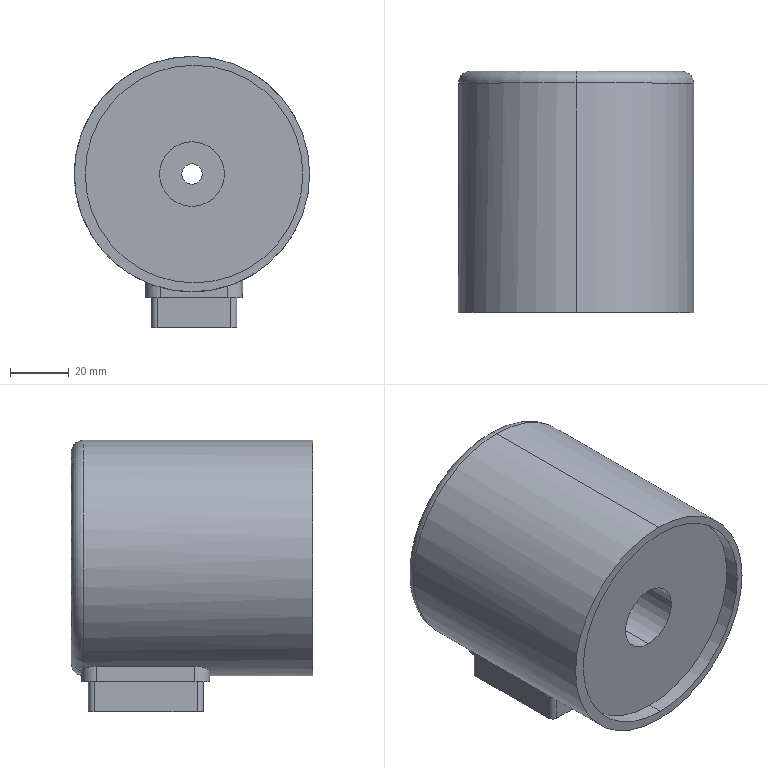Part | STEP file | 1 solid | 36 faces | box 80 x 82 x 92.2 mm | volume 393243 mm3 | cylinder 18 | plane 16 | torus 2 | commonest cylinder face diameters 4 x4 10 x4 80 x4 7 x2 22 x2 74 x2
STEP:
#1=CARTESIAN_POINT('',(0.,-31.446,37.));
#2=VERTEX_POINT('',#1);
#3=CARTESIAN_POINT('',(0.,-31.446,-37.));
#4=VERTEX_POINT('',#3);
#5=CARTESIAN_POINT('',(0.,-31.446,0.));
#6=DIRECTION('',(0.,-1.,0.));
#7=DIRECTION('',(0.,0.,-1.));
#8=AXIS2_PLACEMENT_3D('',#5,#6,#7);
#9=CIRCLE('',#8,37.);
#10=EDGE_CURVE('',#2,#4,#9,.T.);
#11=ORIENTED_EDGE('',*,*,#10,.F.);
#12=CARTESIAN_POINT('',(0.,-36.446,37.));
#13=VERTEX_POINT('',#12);
#14=CARTESIAN_POINT('',(0.,-31.446,37.));
#15=DIRECTION('',(0.,-1.,0.));
#16=VECTOR('',#15,1000.);
#17=LINE('',#14,#16);
#18=EDGE_CURVE('',#2,#13,#17,.T.);
#19=ORIENTED_EDGE('',*,*,#18,.T.);
#20=CARTESIAN_POINT('',(0.,-36.446,-37.));
#21=VERTEX_POINT('',#20);
#22=CARTESIAN_POINT('',(0.,-36.446,0.));
#23=DIRECTION('',(0.,-1.,0.));
#24=DIRECTION('',(0.,0.,-1.));
#25=AXIS2_PLACEMENT_3D('',#22,#23,#24);
#26=CIRCLE('',#25,37.);
#27=EDGE_CURVE('',#13,#21,#26,.T.);
#28=ORIENTED_EDGE('',*,*,#27,.T.);
#29=CARTESIAN_POINT('',(0.,-31.446,-37.));
#30=DIRECTION('',(0.,-1.,0.));
#31=VECTOR('',#30,1000.);
#32=LINE('',#29,#31);
#33=EDGE_CURVE('',#4,#21,#32,.T.);
#34=ORIENTED_EDGE('',*,*,#33,.F.);
#35=EDGE_LOOP('',(#11,#19,#28,#34));
#36=FACE_OUTER_BOUND('',#35,.T.);
#37=CARTESIAN_POINT('',(0.,-31.446,0.));
#38=DIRECTION('',(0.,-1.,0.));
#39=DIRECTION('',(0.,0.,-1.));
#40=AXIS2_PLACEMENT_3D('',#37,#38,#39);
#41=CYLINDRICAL_SURFACE('',#40,37.);
#42=ADVANCED_FACE('',(#36),#41,.F.);
#43=CARTESIAN_POINT('',(13.564,41.554,-37.37));
#44=VERTEX_POINT('',#43);
#45=CARTESIAN_POINT('',(-0.7,41.554,40.));
#46=VERTEX_POINT('',#45);
#47=CARTESIAN_POINT('',(-0.7,41.554,0.));
#48=DIRECTION('',(0.,-1.,0.));
#49=DIRECTION('',(0.,0.,-1.));
#50=AXIS2_PLACEMENT_3D('',#47,#48,#49);
#51=CIRCLE('',#50,40.);
#52=EDGE_CURVE('',#44,#46,#51,.T.);
#53=ORIENTED_EDGE('',*,*,#52,.T.);
#54=CARTESIAN_POINT('',(-0.7,-36.446,40.));
#55=VERTEX_POINT('',#54);
#56=CARTESIAN_POINT('',(-0.7,-36.446,40.));
#57=DIRECTION('',(0.,-1.,0.));
#58=VECTOR('',#57,1000.);
#59=LINE('',#56,#58);
#60=EDGE_CURVE('',#46,#55,#59,.T.);
#61=ORIENTED_EDGE('',*,*,#60,.T.);
#62=CARTESIAN_POINT('',(-0.7,-36.446,-40.));
#63=VERTEX_POINT('',#62);
#64=CARTESIAN_POINT('',(-0.7,-36.446,0.));
#65=DIRECTION('',(0.,-1.,0.));
#66=DIRECTION('',(0.,0.,-1.));
#67=AXIS2_PLACEMENT_3D('',#64,#65,#66);
#68=CIRCLE('',#67,40.);
#69=EDGE_CURVE('',#63,#55,#68,.T.);
#70=ORIENTED_EDGE('',*,*,#69,.F.);
#71=CARTESIAN_POINT('',(-0.7,-1.446,-40.));
#72=VERTEX_POINT('',#71);
#73=CARTESIAN_POINT('',(-0.7,-36.446,-40.));
#74=DIRECTION('',(0.,-1.,0.));
#75=VECTOR('',#74,1000.);
#76=LINE('',#73,#75);
#77=EDGE_CURVE('',#72,#63,#76,.T.);
#78=ORIENTED_EDGE('',*,*,#77,.F.);
#79=CARTESIAN_POINT('',(11.5,-1.446,-38.094));
#80=VERTEX_POINT('',#79);
#81=CARTESIAN_POINT('',(-0.7,-1.446,0.));
#82=DIRECTION('',(0.,-1.,0.));
#83=DIRECTION('',(1.,0.,0.));
#84=AXIS2_PLACEMENT_3D('',#81,#82,#83);
#85=CIRCLE('',#84,40.);
#86=EDGE_CURVE('',#72,#80,#85,.T.);
#87=ORIENTED_EDGE('',*,*,#86,.T.);
#88=CARTESIAN_POINT('',(16.5,3.554,-36.113));
#89=VERTEX_POINT('',#88);
#90=CARTESIAN_POINT('',(11.5,-1.446,-38.094));
#91=CARTESIAN_POINT('',(12.145,-1.446,-37.888));
#92=CARTESIAN_POINT('',(12.785,-1.321,-37.664));
#93=CARTESIAN_POINT('',(13.528,-1.019,-37.384));
#94=CARTESIAN_POINT('',(13.673,-0.9519,-37.329));
#95=CARTESIAN_POINT('',(13.956,-0.8041,-37.218));
#96=CARTESIAN_POINT('',(14.093,-0.7245,-37.165));
#97=CARTESIAN_POINT('',(14.365,-0.5472,-37.055));
#98=CARTESIAN_POINT('',(14.496,-0.4525,-37.001));
#99=CARTESIAN_POINT('',(14.748,-0.2509,-36.897));
#100=CARTESIAN_POINT('',(14.868,-0.1449,-36.846));
#101=CARTESIAN_POINT('',(15.102,0.08269,-36.746));
#102=CARTESIAN_POINT('',(15.213,0.2015,-36.699));
#103=CARTESIAN_POINT('',(15.37,0.3872,-36.63));
#104=CARTESIAN_POINT('',(15.421,0.4504,-36.608));
#105=CARTESIAN_POINT('',(15.52,0.5792,-36.564));
#106=CARTESIAN_POINT('',(15.566,0.6431,-36.543));
#107=CARTESIAN_POINT('',(15.709,0.8492,-36.48));
#108=CARTESIAN_POINT('',(15.796,0.9903,-36.44));
#109=CARTESIAN_POINT('',(15.956,1.28,-36.367));
#110=CARTESIAN_POINT('',(16.029,1.428,-36.334));
#111=CARTESIAN_POINT('',(16.161,1.736,-36.273));
#112=CARTESIAN_POINT('',(16.219,1.893,-36.246));
#113=CARTESIAN_POINT('',(16.294,2.132,-36.21));
#114=CARTESIAN_POINT('',(16.317,2.212,-36.2));
#115=CARTESIAN_POINT('',(16.359,2.374,-36.18));
#116=CARTESIAN_POINT('',(16.378,2.453,-36.171));
#117=CARTESIAN_POINT('',(16.465,2.873,-36.13));
#118=CARTESIAN_POINT('',(16.5,3.212,-36.113));
#119=CARTESIAN_POINT('',(16.5,3.554,-36.113));
#120=B_SPLINE_CURVE_WITH_KNOTS('',3,(#90,#91,#92,#93,#94,#95,#96,#97,#98,#99,#100,#101,#102,#103,#104,#105,#106,#107,#108,#109,#110,#111,#112,#113,#114,#115,#116,#117,#118,#119),.UNSPECIFIED.,.F.,.F.,(4,2,2,2,2,2,2,2,2,2,2,2,2,2,4),(0.,0.25,0.3125,0.375,0.4375,0.5,0.5625,0.5938,0.625,0.6875,0.75,0.8125,0.8438,0.875,1.),.UNSPECIFIED.);
#121=EDGE_CURVE('',#80,#89,#120,.T.);
#122=ORIENTED_EDGE('',*,*,#121,.T.);
#123=CARTESIAN_POINT('',(16.5,37.,-36.113));
#124=VERTEX_POINT('',#123);
#125=CARTESIAN_POINT('',(16.5,-36.446,-36.113));
#126=DIRECTION('',(0.,1.,0.));
#127=VECTOR('',#126,1000.);
#128=LINE('',#125,#127);
#129=EDGE_CURVE('',#89,#124,#128,.T.);
#130=ORIENTED_EDGE('',*,*,#129,.T.);
#131=CARTESIAN_POINT('',(16.5,37.,-36.113));
#132=CARTESIAN_POINT('',(16.5,37.246,-36.113));
#133=CARTESIAN_POINT('',(16.482,37.49,-36.122));
#134=CARTESIAN_POINT('',(16.429,37.851,-36.147));
#135=CARTESIAN_POINT('',(16.395,38.031,-36.163));
#136=CARTESIAN_POINT('',(16.352,38.21,-36.183));
#137=CARTESIAN_POINT('',(16.321,38.328,-36.198));
#138=CARTESIAN_POINT('',(16.304,38.389,-36.206));
#139=CARTESIAN_POINT('',(16.216,38.678,-36.247));
#140=CARTESIAN_POINT('',(16.13,38.903,-36.287));
#141=CARTESIAN_POINT('',(15.978,39.229,-36.357));
#142=CARTESIAN_POINT('',(15.895,39.389,-36.395));
#143=CARTESIAN_POINT('',(15.804,39.546,-36.437));
#144=CARTESIAN_POINT('',(15.741,39.649,-36.465));
#145=CARTESIAN_POINT('',(15.708,39.702,-36.48));
#146=CARTESIAN_POINT('',(15.545,39.949,-36.553));
#147=CARTESIAN_POINT('',(15.401,40.136,-36.617));
#148=CARTESIAN_POINT('',(15.168,40.401,-36.718));
#149=CARTESIAN_POINT('',(15.046,40.529,-36.771));
#150=CARTESIAN_POINT('',(14.917,40.651,-36.825));
#151=CARTESIAN_POINT('',(14.83,40.731,-36.862));
#152=CARTESIAN_POINT('',(14.784,40.771,-36.882));
#153=CARTESIAN_POINT('',(14.383,41.112,-37.049));
#154=CARTESIAN_POINT('',(13.992,41.36,-37.207));
#155=CARTESIAN_POINT('',(13.564,41.554,-37.37));
#156=B_SPLINE_CURVE_WITH_KNOTS('',3,(#131,#132,#133,#134,#135,#136,#137,#138,#139,#140,#141,#142,#143,#144,#145,#146,#147,#148,#149,#150,#151,#152,#153,#154,#155),.UNSPECIFIED.,.F.,.F.,(4,2,1,2,2,2,1,2,2,2,1,2,2,4),(0.,0.125,0.1875,0.2188,0.25,0.375,0.4375,0.4688,0.5,0.625,0.6875,0.7188,0.75,1.),.UNSPECIFIED.);
#157=EDGE_CURVE('',#124,#44,#156,.T.);
#158=ORIENTED_EDGE('',*,*,#157,.T.);
#159=EDGE_LOOP('',(#53,#61,#70,#78,#87,#122,#130,#158));
#160=FACE_OUTER_BOUND('',#159,.T.);
#161=CARTESIAN_POINT('',(-0.7,-36.446,0.));
#162=DIRECTION('',(0.,-1.,0.));
#163=DIRECTION('',(0.,0.,-1.));
#164=AXIS2_PLACEMENT_3D('',#161,#162,#163);
#165=CYLINDRICAL_SURFACE('',#164,40.);
#166=ADVANCED_FACE('',(#160),#165,.T.);
#167=CARTESIAN_POINT('',(-0.7,45.554,-36.));
#168=VERTEX_POINT('',#167);
#169=CARTESIAN_POINT('',(-0.7,45.554,36.));
#170=VERTEX_POINT('',#169);
#171=CARTESIAN_POINT('',(-0.7,45.554,0.));
#172=DIRECTION('',(0.,-1.,0.));
#173=DIRECTION('',(0.,0.,-1.));
#174=AXIS2_PLACEMENT_3D('',#171,#172,#173);
#175=CIRCLE('',#174,36.);
#176=EDGE_CURVE('',#168,#170,#175,.T.);
#177=ORIENTED_EDGE('',*,*,#176,.T.);
#178=CARTESIAN_POINT('',(-0.7,41.554,36.));
#179=DIRECTION('',(1.,0.,0.));
#180=DIRECTION('',(0.,0.,-1.));
#181=AXIS2_PLACEMENT_3D('',#178,#179,#180);
#182=CIRCLE('',#181,4.);
#183=EDGE_CURVE('',#170,#46,#182,.T.);
#184=ORIENTED_EDGE('',*,*,#183,.T.);
#185=ORIENTED_EDGE('',*,*,#52,.F.);
#186=CARTESIAN_POINT('',(11.79,41.554,-38.));
#187=VERTEX_POINT('',#186);
#188=CARTESIAN_POINT('',(-0.7,41.554,0.));
#189=DIRECTION('',(0.,-1.,0.));
#190=DIRECTION('',(0.,0.,-1.));
#191=AXIS2_PLACEMENT_3D('',#188,#189,#190);
#192=CIRCLE('',#191,40.);
#193=EDGE_CURVE('',#187,#44,#192,.T.);
#194=ORIENTED_EDGE('',*,*,#193,.F.);
#195=CARTESIAN_POINT('',(11.711,41.996,-38.));
#196=VERTEX_POINT('',#195);
#197=CARTESIAN_POINT('',(11.711,41.996,-38.));
#198=CARTESIAN_POINT('',(11.737,41.925,-38.));
#199=CARTESIAN_POINT('',(11.756,41.853,-38.));
#200=CARTESIAN_POINT('',(11.783,41.703,-38.));
#201=CARTESIAN_POINT('',(11.79,41.629,-38.));
#202=CARTESIAN_POINT('',(11.79,41.554,-38.));
#203=B_SPLINE_CURVE_WITH_KNOTS('',3,(#197,#198,#199,#200,#201,#202),.UNSPECIFIED.,.F.,.F.,(4,2,4),(0.01192,0.01214,0.01237),.UNSPECIFIED.);
#204=EDGE_CURVE('',#196,#187,#203,.T.);
#205=ORIENTED_EDGE('',*,*,#204,.F.);
#206=CARTESIAN_POINT('',(11.5,42.,-38.068));
#207=VERTEX_POINT('',#206);
#208=CARTESIAN_POINT('',(11.711,41.996,-38.));
#209=CARTESIAN_POINT('',(11.641,41.999,-38.023));
#210=CARTESIAN_POINT('',(11.571,42.,-38.045));
#211=CARTESIAN_POINT('',(11.5,42.,-38.068));
#212=B_SPLINE_CURVE_WITH_KNOTS('',3,(#208,#209,#210,#211),.UNSPECIFIED.,.F.,.F.,(4,4),(0.000000653,0.0002228),.UNSPECIFIED.);
#213=EDGE_CURVE('',#196,#207,#212,.T.);
#214=ORIENTED_EDGE('',*,*,#213,.T.);
#215=CARTESIAN_POINT('',(-0.7,42.,-39.975));
#216=VERTEX_POINT('',#215);
#217=CARTESIAN_POINT('',(-0.7,42.,0.));
#218=DIRECTION('',(0.,1.,0.));
#219=DIRECTION('',(0.,0.,-1.));
#220=AXIS2_PLACEMENT_3D('',#217,#218,#219);
#221=CIRCLE('',#220,39.975);
#222=EDGE_CURVE('',#207,#216,#221,.T.);
#223=ORIENTED_EDGE('',*,*,#222,.T.);
#224=CARTESIAN_POINT('',(-0.7,41.554,-36.));
#225=DIRECTION('',(-1.,0.,0.));
#226=DIRECTION('',(0.,0.,1.));
#227=AXIS2_PLACEMENT_3D('',#224,#225,#226);
#228=CIRCLE('',#227,4.);
#229=EDGE_CURVE('',#168,#216,#228,.T.);
#230=ORIENTED_EDGE('',*,*,#229,.F.);
#231=EDGE_LOOP('',(#177,#184,#185,#194,#205,#214,#223,#230));
#232=FACE_OUTER_BOUND('',#231,.T.);
#233=CARTESIAN_POINT('',(-0.7,41.554,0.));
#234=DIRECTION('',(0.,-1.,0.));
#235=DIRECTION('',(0.,0.,-1.));
#236=AXIS2_PLACEMENT_3D('',#233,#234,#235);
#237=TOROIDAL_SURFACE('',#236,36.,4.);
#238=ADVANCED_FACE('',(#232),#237,.T.);
#239=CARTESIAN_POINT('',(2.8,-3.446,0.));
#240=VERTEX_POINT('',#239);
#241=CARTESIAN_POINT('',(-4.2,-3.446,0.));
#242=VERTEX_POINT('',#241);
#243=CARTESIAN_POINT('',(-0.7,-3.446,0.));
#244=DIRECTION('',(0.,1.,0.));
#245=DIRECTION('',(0.,0.,-1.));
#246=AXIS2_PLACEMENT_3D('',#243,#244,#245);
#247=CIRCLE('',#246,3.5);
#248=EDGE_CURVE('',#240,#242,#247,.T.);
#249=ORIENTED_EDGE('',*,*,#248,.F.);
#250=CARTESIAN_POINT('',(2.8,45.554,0.));
#251=VERTEX_POINT('',#250);
#252=CARTESIAN_POINT('',(2.8,-60.446,0.));
#253=DIRECTION('',(0.,1.,0.));
#254=VECTOR('',#253,1000.);
#255=LINE('',#252,#254);
#256=EDGE_CURVE('',#240,#251,#255,.T.);
#257=ORIENTED_EDGE('',*,*,#256,.T.);
#258=CARTESIAN_POINT('',(-4.2,45.554,0.));
#259=VERTEX_POINT('',#258);
#260=CARTESIAN_POINT('',(-0.7,45.554,0.));
#261=DIRECTION('',(0.,1.,0.));
#262=DIRECTION('',(-1.,0.,0.));
#263=AXIS2_PLACEMENT_3D('',#260,#261,#262);
#264=CIRCLE('',#263,3.5);
#265=EDGE_CURVE('',#251,#259,#264,.T.);
#266=ORIENTED_EDGE('',*,*,#265,.T.);
#267=CARTESIAN_POINT('',(-4.2,-60.446,0.));
#268=DIRECTION('',(0.,1.,0.));
#269=VECTOR('',#268,1000.);
#270=LINE('',#267,#269);
#271=EDGE_CURVE('',#242,#259,#270,.T.);
#272=ORIENTED_EDGE('',*,*,#271,.F.);
#273=EDGE_LOOP('',(#249,#257,#266,#272));
#274=FACE_OUTER_BOUND('',#273,.T.);
#275=CARTESIAN_POINT('',(-0.7,-60.446,0.));
#276=DIRECTION('',(0.,1.,0.));
#277=DIRECTION('',(-1.,0.,0.));
#278=AXIS2_PLACEMENT_3D('',#275,#276,#277);
#279=CYLINDRICAL_SURFACE('',#278,3.5);
#280=ADVANCED_FACE('',(#274),#279,.F.);
#281=CARTESIAN_POINT('',(-0.7,-3.446,11.));
#282=VERTEX_POINT('',#281);
#283=CARTESIAN_POINT('',(-0.7,-3.446,-11.));
#284=VERTEX_POINT('',#283);
#285=CARTESIAN_POINT('',(-0.7,-3.446,0.));
#286=DIRECTION('',(0.,-1.,0.));
#287=DIRECTION('',(0.,0.,-1.));
#288=AXIS2_PLACEMENT_3D('',#285,#286,#287);
#289=CIRCLE('',#288,11.);
#290=EDGE_CURVE('',#282,#284,#289,.T.);
#291=ORIENTED_EDGE('',*,*,#290,.F.);
#292=CARTESIAN_POINT('',(-0.7,-31.446,11.));
#293=VERTEX_POINT('',#292);
#294=CARTESIAN_POINT('',(-0.7,-3.446,11.));
#295=DIRECTION('',(0.,-1.,0.));
#296=VECTOR('',#295,1000.);
#297=LINE('',#294,#296);
#298=EDGE_CURVE('',#282,#293,#297,.T.);
#299=ORIENTED_EDGE('',*,*,#298,.T.);
#300=CARTESIAN_POINT('',(-0.7,-31.446,-11.));
#301=VERTEX_POINT('',#300);
#302=CARTESIAN_POINT('',(-0.7,-31.446,0.));
#303=DIRECTION('',(0.,1.,0.));
#304=DIRECTION('',(0.,0.,-1.));
#305=AXIS2_PLACEMENT_3D('',#302,#303,#304);
#306=CIRCLE('',#305,11.);
#307=EDGE_CURVE('',#301,#293,#306,.T.);
#308=ORIENTED_EDGE('',*,*,#307,.F.);
#309=CARTESIAN_POINT('',(-0.7,-3.446,-11.));
#310=DIRECTION('',(0.,-1.,0.));
#311=VECTOR('',#310,1000.);
#312=LINE('',#309,#311);
#313=EDGE_CURVE('',#284,#301,#312,.T.);
#314=ORIENTED_EDGE('',*,*,#313,.F.);
#315=EDGE_LOOP('',(#291,#299,#308,#314));
#316=FACE_OUTER_BOUND('',#315,.T.);
#317=CARTESIAN_POINT('',(-0.7,-3.446,0.));
#318=DIRECTION('',(0.,-1.,0.));
#319=DIRECTION('',(0.,0.,-1.));
#320=AXIS2_PLACEMENT_3D('',#317,#318,#319);
#321=CYLINDRICAL_SURFACE('',#320,11.);
#322=ADVANCED_FACE('',(#316),#321,.F.);
#323=CARTESIAN_POINT('',(16.5,37.,-42.));
#324=VERTEX_POINT('',#323);
#325=CARTESIAN_POINT('',(16.5,3.554,-42.));
#326=VERTEX_POINT('',#325);
#327=CARTESIAN_POINT('',(16.5,3.554,-42.));
#328=DIRECTION('',(0.,-1.,0.));
#329=VECTOR('',#328,1000.);
#330=LINE('',#327,#329);
#331=EDGE_CURVE('',#324,#326,#330,.T.);
#332=ORIENTED_EDGE('',*,*,#331,.T.);
#333=CARTESIAN_POINT('',(11.5,-1.446,-42.));
#334=VERTEX_POINT('',#333);
#335=CARTESIAN_POINT('',(11.5,3.554,-42.));
#336=DIRECTION('',(0.,0.,-1.));
#337=DIRECTION('',(1.,0.,0.));
#338=AXIS2_PLACEMENT_3D('',#335,#336,#337);
#339=CIRCLE('',#338,5.);
#340=EDGE_CURVE('',#326,#334,#339,.T.);
#341=ORIENTED_EDGE('',*,*,#340,.T.);
#342=CARTESIAN_POINT('',(-11.5,-1.446,-42.));
#343=VERTEX_POINT('',#342);
#344=CARTESIAN_POINT('',(11.5,-1.446,-42.));
#345=DIRECTION('',(-1.,0.,0.));
#346=VECTOR('',#345,1000.);
#347=LINE('',#344,#346);
#348=EDGE_CURVE('',#334,#343,#347,.T.);
#349=ORIENTED_EDGE('',*,*,#348,.T.);
#350=CARTESIAN_POINT('',(-16.5,3.554,-42.));
#351=VERTEX_POINT('',#350);
#352=CARTESIAN_POINT('',(-11.5,3.554,-42.));
#353=DIRECTION('',(0.,0.,-1.));
#354=DIRECTION('',(1.,0.,0.));
#355=AXIS2_PLACEMENT_3D('',#352,#353,#354);
#356=CIRCLE('',#355,5.);
#357=EDGE_CURVE('',#343,#351,#356,.T.);
#358=ORIENTED_EDGE('',*,*,#357,.T.);
#359=CARTESIAN_POINT('',(-16.5,37.,-42.));
#360=VERTEX_POINT('',#359);
#361=CARTESIAN_POINT('',(-16.5,37.,-42.));
#362=DIRECTION('',(0.,1.,0.));
#363=VECTOR('',#362,1000.);
#364=LINE('',#361,#363);
#365=EDGE_CURVE('',#351,#360,#364,.T.);
#366=ORIENTED_EDGE('',*,*,#365,.T.);
#367=CARTESIAN_POINT('',(-11.5,42.,-42.));
#368=VERTEX_POINT('',#367);
#369=CARTESIAN_POINT('',(-11.5,37.,-42.));
#370=DIRECTION('',(0.,0.,-1.));
#371=DIRECTION('',(1.,0.,0.));
#372=AXIS2_PLACEMENT_3D('',#369,#370,#371);
#373=CIRCLE('',#372,5.);
#374=EDGE_CURVE('',#360,#368,#373,.T.);
#375=ORIENTED_EDGE('',*,*,#374,.T.);
#376=CARTESIAN_POINT('',(11.5,42.,-42.));
#377=VERTEX_POINT('',#376);
#378=CARTESIAN_POINT('',(-11.5,42.,-42.));
#379=DIRECTION('',(1.,0.,0.));
#380=VECTOR('',#379,1000.);
#381=LINE('',#378,#380);
#382=EDGE_CURVE('',#368,#377,#381,.T.);
#383=ORIENTED_EDGE('',*,*,#382,.T.);
#384=CARTESIAN_POINT('',(11.5,37.,-42.));
#385=DIRECTION('',(0.,0.,-1.));
#386=DIRECTION('',(1.,0.,0.));
#387=AXIS2_PLACEMENT_3D('',#384,#385,#386);
#388=CIRCLE('',#387,5.);
#389=EDGE_CURVE('',#377,#324,#388,.T.);
#390=ORIENTED_EDGE('',*,*,#389,.T.);
#391=EDGE_LOOP('',(#332,#341,#349,#358,#366,#375,#383,#390));
#392=FACE_OUTER_BOUND('',#391,.T.);
#393=CARTESIAN_POINT('',(-12.5,0.777,-42.));
#394=VERTEX_POINT('',#393);
#395=CARTESIAN_POINT('',(-14.5,2.777,-42.));
#396=VERTEX_POINT('',#395);
#397=CARTESIAN_POINT('',(-12.5,2.777,-42.));
#398=DIRECTION('',(0.,0.,-1.));
#399=DIRECTION('',(-1.,0.,0.));
#400=AXIS2_PLACEMENT_3D('',#397,#398,#399);
#401=CIRCLE('',#400,2.);
#402=EDGE_CURVE('',#394,#396,#401,.T.);
#403=ORIENTED_EDGE('',*,*,#402,.F.);
#404=CARTESIAN_POINT('',(12.5,0.777,-42.));
#405=VERTEX_POINT('',#404);
#406=CARTESIAN_POINT('',(12.5,0.777,-42.));
#407=DIRECTION('',(-1.,0.,0.));
#408=VECTOR('',#407,1000.);
#409=LINE('',#406,#408);
#410=EDGE_CURVE('',#405,#394,#409,.T.);
#411=ORIENTED_EDGE('',*,*,#410,.F.);
#412=CARTESIAN_POINT('',(14.5,2.777,-42.));
#413=VERTEX_POINT('',#412);
#414=CARTESIAN_POINT('',(12.5,2.777,-42.));
#415=DIRECTION('',(0.,0.,-1.));
#416=DIRECTION('',(1.,0.,0.));
#417=AXIS2_PLACEMENT_3D('',#414,#415,#416);
#418=CIRCLE('',#417,2.);
#419=EDGE_CURVE('',#413,#405,#418,.T.);
#420=ORIENTED_EDGE('',*,*,#419,.F.);
#421=CARTESIAN_POINT('',(14.5,37.777,-42.));
#422=VERTEX_POINT('',#421);
#423=CARTESIAN_POINT('',(14.5,2.777,-42.));
#424=DIRECTION('',(0.,-1.,0.));
#425=VECTOR('',#424,1000.);
#426=LINE('',#423,#425);
#427=EDGE_CURVE('',#422,#413,#426,.T.);
#428=ORIENTED_EDGE('',*,*,#427,.F.);
#429=CARTESIAN_POINT('',(12.5,39.777,-42.));
#430=VERTEX_POINT('',#429);
#431=CARTESIAN_POINT('',(12.5,37.777,-42.));
#432=DIRECTION('',(0.,0.,-1.));
#433=DIRECTION('',(1.,0.,0.));
#434=AXIS2_PLACEMENT_3D('',#431,#432,#433);
#435=CIRCLE('',#434,2.);
#436=EDGE_CURVE('',#430,#422,#435,.T.);
#437=ORIENTED_EDGE('',*,*,#436,.F.);
#438=CARTESIAN_POINT('',(-12.5,39.777,-42.));
#439=VERTEX_POINT('',#438);
#440=CARTESIAN_POINT('',(12.5,39.777,-42.));
#441=DIRECTION('',(1.,0.,0.));
#442=VECTOR('',#441,1000.);
#443=LINE('',#440,#442);
#444=EDGE_CURVE('',#439,#430,#443,.T.);
#445=ORIENTED_EDGE('',*,*,#444,.F.);
#446=CARTESIAN_POINT('',(-14.5,37.777,-42.));
#447=VERTEX_POINT('',#446);
#448=CARTESIAN_POINT('',(-12.5,37.777,-42.));
#449=DIRECTION('',(0.,0.,-1.));
#450=DIRECTION('',(1.,0.,0.));
#451=AXIS2_PLACEMENT_3D('',#448,#449,#450);
#452=CIRCLE('',#451,2.);
#453=EDGE_CURVE('',#447,#439,#452,.T.);
#454=ORIENTED_EDGE('',*,*,#453,.F.);
#455=CARTESIAN_POINT('',(-14.5,2.777,-42.));
#456=DIRECTION('',(0.,1.,0.));
#457=VECTOR('',#456,1000.);
#458=LINE('',#455,#457);
#459=EDGE_CURVE('',#396,#447,#458,.T.);
#460=ORIENTED_EDGE('',*,*,#459,.F.);
#461=EDGE_LOOP('',(#403,#411,#420,#428,#437,#445,#454,#460));
#462=FACE_BOUND('',#461,.T.);
#463=CARTESIAN_POINT('',(11.5,37.,-42.));
#464=DIRECTION('',(0.,0.,1.));
#465=DIRECTION('',(1.,0.,0.));
#466=AXIS2_PLACEMENT_3D('',#463,#464,#465);
#467=PLANE('',#466);
#468=ADVANCED_FACE('',(#392,#462),#467,.F.);
#469=ORIENTED_EDGE('',*,*,#298,.F.);
#470=CARTESIAN_POINT('',(-0.7,-3.446,0.));
#471=DIRECTION('',(0.,-1.,0.));
#472=DIRECTION('',(0.,0.,-1.));
#473=AXIS2_PLACEMENT_3D('',#470,#471,#472);
#474=CIRCLE('',#473,11.);
#475=EDGE_CURVE('',#284,#282,#474,.T.);
#476=ORIENTED_EDGE('',*,*,#475,.F.);
#477=ORIENTED_EDGE('',*,*,#313,.T.);
#478=CARTESIAN_POINT('',(-0.7,-31.446,0.));
#479=DIRECTION('',(0.,1.,0.));
#480=DIRECTION('',(0.,0.,-1.));
#481=AXIS2_PLACEMENT_3D('',#478,#479,#480);
#482=CIRCLE('',#481,11.);
#483=EDGE_CURVE('',#293,#301,#482,.T.);
#484=ORIENTED_EDGE('',*,*,#483,.F.);
#485=EDGE_LOOP('',(#469,#476,#477,#484));
#486=FACE_OUTER_BOUND('',#485,.T.);
#487=CARTESIAN_POINT('',(-0.7,-3.446,0.));
#488=DIRECTION('',(0.,-1.,0.));
#489=DIRECTION('',(0.,0.,-1.));
#490=AXIS2_PLACEMENT_3D('',#487,#488,#489);
#491=CYLINDRICAL_SURFACE('',#490,11.);
#492=ADVANCED_FACE('',(#486),#491,.F.);
#493=ORIENTED_EDGE('',*,*,#256,.F.);
#494=CARTESIAN_POINT('',(-0.7,-3.446,0.));
#495=DIRECTION('',(0.,1.,0.));
#496=DIRECTION('',(0.,0.,-1.));
#497=AXIS2_PLACEMENT_3D('',#494,#495,#496);
#498=CIRCLE('',#497,3.5);
#499=EDGE_CURVE('',#242,#240,#498,.T.);
#500=ORIENTED_EDGE('',*,*,#499,.F.);
#501=ORIENTED_EDGE('',*,*,#271,.T.);
#502=CARTESIAN_POINT('',(-0.7,45.554,0.));
#503=DIRECTION('',(0.,1.,0.));
#504=DIRECTION('',(-1.,0.,0.));
#505=AXIS2_PLACEMENT_3D('',#502,#503,#504);
#506=CIRCLE('',#505,3.5);
#507=EDGE_CURVE('',#259,#251,#506,.T.);
#508=ORIENTED_EDGE('',*,*,#507,.T.);
#509=EDGE_LOOP('',(#493,#500,#501,#508));
#510=FACE_OUTER_BOUND('',#509,.T.);
#511=CARTESIAN_POINT('',(-0.7,-60.446,0.));
#512=DIRECTION('',(0.,1.,0.));
#513=DIRECTION('',(-1.,0.,0.));
#514=AXIS2_PLACEMENT_3D('',#511,#512,#513);
#515=CYLINDRICAL_SURFACE('',#514,3.5);
#516=ADVANCED_FACE('',(#510),#515,.F.);
#517=CARTESIAN_POINT('',(-13.564,41.554,-37.875));
#518=VERTEX_POINT('',#517);
#519=CARTESIAN_POINT('',(-13.19,41.554,-38.));
#520=VERTEX_POINT('',#519);
#521=CARTESIAN_POINT('',(-0.7,41.554,0.));
#522=DIRECTION('',(0.,-1.,0.));
#523=DIRECTION('',(0.,0.,-1.));
#524=AXIS2_PLACEMENT_3D('',#521,#522,#523);
#525=CIRCLE('',#524,40.);
#526=EDGE_CURVE('',#518,#520,#525,.T.);
#527=ORIENTED_EDGE('',*,*,#526,.T.);
#528=CARTESIAN_POINT('',(-13.19,41.706,-38.));
#529=VERTEX_POINT('',#528);
#530=CARTESIAN_POINT('',(-13.19,-36.446,-38.));
#531=DIRECTION('',(0.,1.,0.));
#532=VECTOR('',#531,1000.);
#533=LINE('',#530,#532);
#534=EDGE_CURVE('',#520,#529,#533,.T.);
#535=ORIENTED_EDGE('',*,*,#534,.T.);
#536=CARTESIAN_POINT('',(-13.19,41.706,-38.));
#537=CARTESIAN_POINT('',(-13.317,41.66,-37.958));
#538=CARTESIAN_POINT('',(-13.442,41.609,-37.916));
#539=CARTESIAN_POINT('',(-13.564,41.554,-37.875));
#540=B_SPLINE_CURVE_WITH_KNOTS('',3,(#536,#537,#538,#539),.UNSPECIFIED.,.F.,.F.,(4,4),(0.001791,0.00221),.UNSPECIFIED.);
#541=EDGE_CURVE('',#529,#518,#540,.T.);
#542=ORIENTED_EDGE('',*,*,#541,.T.);
#543=EDGE_LOOP('',(#527,#535,#542));
#544=FACE_OUTER_BOUND('',#543,.T.);
#545=CARTESIAN_POINT('',(-0.7,-36.446,0.));
#546=DIRECTION('',(0.,-1.,0.));
#547=DIRECTION('',(0.,0.,-1.));
#548=AXIS2_PLACEMENT_3D('',#545,#546,#547);
#549=CYLINDRICAL_SURFACE('',#548,40.);
#550=ADVANCED_FACE('',(#544),#549,.F.);
#551=ORIENTED_EDGE('',*,*,#176,.F.);
#552=CARTESIAN_POINT('',(-0.7,45.554,0.));
#553=DIRECTION('',(0.,-1.,0.));
#554=DIRECTION('',(0.,0.,-1.));
#555=AXIS2_PLACEMENT_3D('',#552,#553,#554);
#556=CIRCLE('',#555,36.);
#557=EDGE_CURVE('',#170,#168,#556,.T.);
#558=ORIENTED_EDGE('',*,*,#557,.F.);
#559=EDGE_LOOP('',(#551,#558));
#560=FACE_OUTER_BOUND('',#559,.T.);
#561=ORIENTED_EDGE('',*,*,#507,.F.);
#562=ORIENTED_EDGE('',*,*,#265,.F.);
#563=EDGE_LOOP('',(#561,#562));
#564=FACE_BOUND('',#563,.T.);
#565=CARTESIAN_POINT('',(-0.7,45.554,0.));
#566=DIRECTION('',(0.,1.,0.));
#567=DIRECTION('',(1.,0.,0.));
#568=AXIS2_PLACEMENT_3D('',#565,#566,#567);
#569=PLANE('',#568);
#570=ADVANCED_FACE('',(#560,#564),#569,.T.);
#571=ORIENTED_EDGE('',*,*,#183,.F.);
#572=ORIENTED_EDGE('',*,*,#557,.T.);
#573=ORIENTED_EDGE('',*,*,#229,.T.);
#574=CARTESIAN_POINT('',(-11.5,42.,-38.489));
#575=VERTEX_POINT('',#574);
#576=CARTESIAN_POINT('',(-0.7,42.,0.));
#577=DIRECTION('',(0.,1.,0.));
#578=DIRECTION('',(0.,0.,-1.));
#579=AXIS2_PLACEMENT_3D('',#576,#577,#578);
#580=CIRCLE('',#579,39.975);
#581=EDGE_CURVE('',#216,#575,#580,.T.);
#582=ORIENTED_EDGE('',*,*,#581,.T.);
#583=CARTESIAN_POINT('',(-13.18,41.709,-38.));
#584=VERTEX_POINT('',#583);
#585=CARTESIAN_POINT('',(-11.5,42.,-38.489));
#586=CARTESIAN_POINT('',(-12.074,42.,-38.328));
#587=CARTESIAN_POINT('',(-12.636,41.904,-38.171));
#588=CARTESIAN_POINT('',(-13.18,41.709,-38.));
#589=B_SPLINE_CURVE_WITH_KNOTS('',3,(#585,#586,#587,#588),.UNSPECIFIED.,.F.,.F.,(4,4),(0.,1.),.UNSPECIFIED.);
#590=EDGE_CURVE('',#575,#584,#589,.T.);
#591=ORIENTED_EDGE('',*,*,#590,.T.);
#592=CARTESIAN_POINT('',(-13.19,41.554,-38.));
#593=CARTESIAN_POINT('',(-13.19,41.58,-38.));
#594=CARTESIAN_POINT('',(-13.188,41.632,-38.));
#595=CARTESIAN_POINT('',(-13.184,41.683,-38.));
#596=CARTESIAN_POINT('',(-13.18,41.709,-38.));
#597=B_SPLINE_CURVE_WITH_KNOTS('',3,(#592,#593,#594,#595,#596),.UNSPECIFIED.,.F.,.F.,(4,1,4),(0.03968,0.03975,0.03983),.UNSPECIFIED.);
#598=EDGE_CURVE('',#520,#584,#597,.T.);
#599=ORIENTED_EDGE('',*,*,#598,.F.);
#600=ORIENTED_EDGE('',*,*,#526,.F.);
#601=CARTESIAN_POINT('',(-0.7,41.554,0.));
#602=DIRECTION('',(0.,-1.,0.));
#603=DIRECTION('',(0.,0.,-1.));
#604=AXIS2_PLACEMENT_3D('',#601,#602,#603);
#605=CIRCLE('',#604,40.);
#606=EDGE_CURVE('',#46,#518,#605,.T.);
#607=ORIENTED_EDGE('',*,*,#606,.F.);
#608=EDGE_LOOP('',(#571,#572,#573,#582,#591,#599,#600,#607));
#609=FACE_OUTER_BOUND('',#608,.T.);
#610=CARTESIAN_POINT('',(-0.7,41.554,0.));
#611=DIRECTION('',(0.,-1.,0.));
#612=DIRECTION('',(0.,0.,-1.));
#613=AXIS2_PLACEMENT_3D('',#610,#611,#612);
#614=TOROIDAL_SURFACE('',#613,36.,4.);
#615=ADVANCED_FACE('',(#609),#614,.T.);
#616=ORIENTED_EDGE('',*,*,#60,.F.);
#617=ORIENTED_EDGE('',*,*,#606,.T.);
#618=CARTESIAN_POINT('',(-16.5,37.,-36.747));
#619=VERTEX_POINT('',#618);
#620=CARTESIAN_POINT('',(-16.5,37.,-36.747));
#621=CARTESIAN_POINT('',(-16.5,37.24,-36.747));
#622=CARTESIAN_POINT('',(-16.483,37.481,-36.755));
#623=CARTESIAN_POINT('',(-16.43,37.842,-36.777));
#624=CARTESIAN_POINT('',(-16.408,37.963,-36.787));
#625=CARTESIAN_POINT('',(-16.368,38.142,-36.804));
#626=CARTESIAN_POINT('',(-16.347,38.232,-36.813));
#627=CARTESIAN_POINT('',(-16.318,38.336,-36.825));
#628=CARTESIAN_POINT('',(-16.306,38.38,-36.83));
#629=CARTESIAN_POINT('',(-16.297,38.41,-36.834));
#630=CARTESIAN_POINT('',(-16.292,38.426,-36.836));
#631=CARTESIAN_POINT('',(-16.222,38.658,-36.865));
#632=CARTESIAN_POINT('',(-16.14,38.879,-36.9));
#633=CARTESIAN_POINT('',(-15.989,39.206,-36.963));
#634=CARTESIAN_POINT('',(-15.934,39.315,-36.986));
#635=CARTESIAN_POINT('',(-15.844,39.476,-37.022));
#636=CARTESIAN_POINT('',(-15.798,39.557,-37.041));
#637=CARTESIAN_POINT('',(-15.74,39.65,-37.065));
#638=CARTESIAN_POINT('',(-15.711,39.696,-37.077));
#639=CARTESIAN_POINT('',(-15.698,39.716,-37.082));
#640=CARTESIAN_POINT('',(-15.69,39.729,-37.085));
#641=CARTESIAN_POINT('',(-15.685,39.737,-37.087));
#642=CARTESIAN_POINT('',(-15.564,39.92,-37.136));
#643=CARTESIAN_POINT('',(-15.43,40.1,-37.19));
#644=CARTESIAN_POINT('',(-15.197,40.368,-37.281));
#645=CARTESIAN_POINT('',(-15.115,40.457,-37.313));
#646=CARTESIAN_POINT('',(-14.983,40.588,-37.363));
#647=CARTESIAN_POINT('',(-14.915,40.654,-37.389));
#648=CARTESIAN_POINT('',(-14.832,40.729,-37.421));
#649=CARTESIAN_POINT('',(-14.789,40.766,-37.437));
#650=CARTESIAN_POINT('',(-14.768,40.784,-37.445));
#651=CARTESIAN_POINT('',(-14.759,40.792,-37.448));
#652=CARTESIAN_POINT('',(-14.752,40.798,-37.45));
#653=CARTESIAN_POINT('',(-14.748,40.801,-37.452));
#654=CARTESIAN_POINT('',(-14.616,40.914,-37.502));
#655=CARTESIAN_POINT('',(-14.456,41.04,-37.561));
#656=CARTESIAN_POINT('',(-14.065,41.298,-37.702));
#657=CARTESIAN_POINT('',(-13.835,41.431,-37.783));
#658=CARTESIAN_POINT('',(-13.564,41.554,-37.875));
#659=B_SPLINE_CURVE_WITH_KNOTS('',3,(#620,#621,#622,#623,#624,#625,#626,#627,#628,#629,#630,#631,#632,#633,#634,#635,#636,#637,#638,#639,#640,#641,#642,#643,#644,#645,#646,#647,#648,#649,#650,#651,#652,#653,#654,#655,#656,#657,#658),.UNSPECIFIED.,.F.,.F.,(4,2,2,1,1,2,2,2,2,1,1,1,2,2,2,2,1,1,1,1,2,2,2,4),(0.,0.125,0.1875,0.2187,0.2344,0.2422,0.25,0.375,0.4375,0.4687,0.4844,0.4922,0.4961,0.5,0.625,0.6875,0.7187,0.7344,0.7422,0.7461,0.748,0.75,0.875,1.),.UNSPECIFIED.);
#660=EDGE_CURVE('',#619,#518,#659,.T.);
#661=ORIENTED_EDGE('',*,*,#660,.F.);
#662=CARTESIAN_POINT('',(-16.5,3.554,-36.747));
#663=VERTEX_POINT('',#662);
#664=CARTESIAN_POINT('',(-16.5,-36.446,-36.747));
#665=DIRECTION('',(0.,-1.,0.));
#666=VECTOR('',#665,1000.);
#667=LINE('',#664,#666);
#668=EDGE_CURVE('',#619,#663,#667,.T.);
#669=ORIENTED_EDGE('',*,*,#668,.T.);
#670=CARTESIAN_POINT('',(-11.5,-1.446,-38.514));
#671=VERTEX_POINT('',#670);
#672=CARTESIAN_POINT('',(-16.5,3.554,-36.747));
#673=CARTESIAN_POINT('',(-16.5,3.217,-36.747));
#674=CARTESIAN_POINT('',(-16.466,2.882,-36.762));
#675=CARTESIAN_POINT('',(-16.365,2.389,-36.805));
#676=CARTESIAN_POINT('',(-16.324,2.227,-36.823));
#677=CARTESIAN_POINT('',(-16.249,1.988,-36.854));
#678=CARTESIAN_POINT('',(-16.222,1.909,-36.865));
#679=CARTESIAN_POINT('',(-16.165,1.752,-36.89));
#680=CARTESIAN_POINT('',(-16.133,1.672,-36.903));
#681=CARTESIAN_POINT('',(-16.036,1.444,-36.943));
#682=CARTESIAN_POINT('',(-15.964,1.296,-36.973));
#683=CARTESIAN_POINT('',(-15.806,1.008,-37.038));
#684=CARTESIAN_POINT('',(-15.719,0.8653,-37.074));
#685=CARTESIAN_POINT('',(-15.534,0.5952,-37.148));
#686=CARTESIAN_POINT('',(-15.435,0.4652,-37.187));
#687=CARTESIAN_POINT('',(-15.226,0.2153,-37.27));
#688=CARTESIAN_POINT('',(-15.113,0.09393,-37.313));
#689=CARTESIAN_POINT('',(-14.881,-0.133,-37.402));
#690=CARTESIAN_POINT('',(-14.76,-0.2405,-37.448));
#691=CARTESIAN_POINT('',(-14.508,-0.4432,-37.541));
#692=CARTESIAN_POINT('',(-14.376,-0.5394,-37.59));
#693=CARTESIAN_POINT('',(-13.972,-0.804,-37.735));
#694=CARTESIAN_POINT('',(-13.69,-0.9525,-37.833));
#695=CARTESIAN_POINT('',(-13.091,-1.197,-38.034));
#696=CARTESIAN_POINT('',(-12.783,-1.289,-38.133));
#697=CARTESIAN_POINT('',(-12.146,-1.415,-38.329));
#698=CARTESIAN_POINT('',(-11.825,-1.446,-38.423));
#699=CARTESIAN_POINT('',(-11.5,-1.446,-38.514));
#700=B_SPLINE_CURVE_WITH_KNOTS('',3,(#672,#673,#674,#675,#676,#677,#678,#679,#680,#681,#682,#683,#684,#685,#686,#687,#688,#689,#690,#691,#692,#693,#694,#695,#696,#697,#698,#699),.UNSPECIFIED.,.F.,.F.,(4,2,2,2,2,2,2,2,2,2,2,2,2,4),(0.,0.125,0.1875,0.2187,0.25,0.3125,0.375,0.4375,0.5,0.5625,0.625,0.75,0.875,1.),.UNSPECIFIED.);
#701=EDGE_CURVE('',#663,#671,#700,.T.);
#702=ORIENTED_EDGE('',*,*,#701,.T.);
#703=CARTESIAN_POINT('',(-0.7,-1.446,0.));
#704=DIRECTION('',(0.,-1.,0.));
#705=DIRECTION('',(1.,0.,0.));
#706=AXIS2_PLACEMENT_3D('',#703,#704,#705);
#707=CIRCLE('',#706,40.);
#708=EDGE_CURVE('',#671,#72,#707,.T.);
#709=ORIENTED_EDGE('',*,*,#708,.T.);
#710=ORIENTED_EDGE('',*,*,#77,.T.);
#711=CARTESIAN_POINT('',(-0.7,-36.446,0.));
#712=DIRECTION('',(0.,-1.,0.));
#713=DIRECTION('',(0.,0.,-1.));
#714=AXIS2_PLACEMENT_3D('',#711,#712,#713);
#715=CIRCLE('',#714,40.);
#716=EDGE_CURVE('',#55,#63,#715,.T.);
#717=ORIENTED_EDGE('',*,*,#716,.F.);
#718=EDGE_LOOP('',(#616,#617,#661,#669,#702,#709,#710,#717));
#719=FACE_OUTER_BOUND('',#718,.T.);
#720=CARTESIAN_POINT('',(-0.7,-36.446,0.));
#721=DIRECTION('',(0.,-1.,0.));
#722=DIRECTION('',(0.,0.,-1.));
#723=AXIS2_PLACEMENT_3D('',#720,#721,#722);
#724=CYLINDRICAL_SURFACE('',#723,40.);
#725=ADVANCED_FACE('',(#719),#724,.T.);
#726=ORIENTED_EDGE('',*,*,#69,.T.);
#727=ORIENTED_EDGE('',*,*,#716,.T.);
#728=EDGE_LOOP('',(#726,#727));
#729=FACE_OUTER_BOUND('',#728,.T.);
#730=CARTESIAN_POINT('',(0.,-36.446,0.));
#731=DIRECTION('',(0.,-1.,0.));
#732=DIRECTION('',(0.,0.,-1.));
#733=AXIS2_PLACEMENT_3D('',#730,#731,#732);
#734=CIRCLE('',#733,37.);
#735=EDGE_CURVE('',#21,#13,#734,.T.);
#736=ORIENTED_EDGE('',*,*,#735,.F.);
#737=ORIENTED_EDGE('',*,*,#27,.F.);
#738=EDGE_LOOP('',(#736,#737));
#739=FACE_BOUND('',#738,.T.);
#740=CARTESIAN_POINT('',(39.3,-36.446,0.));
#741=DIRECTION('',(0.,-1.,0.));
#742=DIRECTION('',(0.,0.,-1.));
#743=AXIS2_PLACEMENT_3D('',#740,#741,#742);
#744=PLANE('',#743);
#745=ADVANCED_FACE('',(#729,#739),#744,.T.);
#746=CARTESIAN_POINT('',(16.5,3.554,40.001));
#747=DIRECTION('',(0.,0.,-1.));
#748=VECTOR('',#747,1000.);
#749=LINE('',#746,#748);
#750=EDGE_CURVE('',#89,#326,#749,.T.);
#751=ORIENTED_EDGE('',*,*,#750,.T.);
#752=ORIENTED_EDGE('',*,*,#331,.F.);
#753=CARTESIAN_POINT('',(16.5,37.,40.001));
#754=DIRECTION('',(0.,0.,-1.));
#755=VECTOR('',#754,1000.);
#756=LINE('',#753,#755);
#757=EDGE_CURVE('',#124,#324,#756,.T.);
#758=ORIENTED_EDGE('',*,*,#757,.F.);
#759=ORIENTED_EDGE('',*,*,#129,.F.);
#760=EDGE_LOOP('',(#751,#752,#758,#759));
#761=FACE_OUTER_BOUND('',#760,.T.);
#762=CARTESIAN_POINT('',(16.5,3.554,40.001));
#763=DIRECTION('',(1.,0.,0.));
#764=DIRECTION('',(0.,1.,0.));
#765=AXIS2_PLACEMENT_3D('',#762,#763,#764);
#766=PLANE('',#765);
#767=ADVANCED_FACE('',(#761),#766,.T.);
#768=ORIENTED_EDGE('',*,*,#121,.F.);
#769=CARTESIAN_POINT('',(11.5,-1.446,40.001));
#770=DIRECTION('',(0.,0.,-1.));
#771=VECTOR('',#770,1000.);
#772=LINE('',#769,#771);
#773=EDGE_CURVE('',#80,#334,#772,.T.);
#774=ORIENTED_EDGE('',*,*,#773,.T.);
#775=ORIENTED_EDGE('',*,*,#340,.F.);
#776=ORIENTED_EDGE('',*,*,#750,.F.);
#777=EDGE_LOOP('',(#768,#774,#775,#776));
#778=FACE_OUTER_BOUND('',#777,.T.);
#779=CARTESIAN_POINT('',(11.5,3.554,40.001));
#780=DIRECTION('',(0.,0.,-1.));
#781=DIRECTION('',(-1.,0.,0.));
#782=AXIS2_PLACEMENT_3D('',#779,#780,#781);
#783=CYLINDRICAL_SURFACE('',#782,5.);
#784=ADVANCED_FACE('',(#778),#783,.T.);
#785=ORIENTED_EDGE('',*,*,#708,.F.);
#786=CARTESIAN_POINT('',(-11.5,-1.446,40.001));
#787=DIRECTION('',(0.,0.,-1.));
#788=VECTOR('',#787,1000.);
#789=LINE('',#786,#788);
#790=EDGE_CURVE('',#671,#343,#789,.T.);
#791=ORIENTED_EDGE('',*,*,#790,.T.);
#792=ORIENTED_EDGE('',*,*,#348,.F.);
#793=ORIENTED_EDGE('',*,*,#773,.F.);
#794=ORIENTED_EDGE('',*,*,#86,.F.);
#795=EDGE_LOOP('',(#785,#791,#792,#793,#794));
#796=FACE_OUTER_BOUND('',#795,.T.);
#797=CARTESIAN_POINT('',(11.5,-1.446,40.001));
#798=DIRECTION('',(0.,-1.,0.));
#799=DIRECTION('',(-1.,0.,0.));
#800=AXIS2_PLACEMENT_3D('',#797,#798,#799);
#801=PLANE('',#800);
#802=ADVANCED_FACE('',(#796),#801,.T.);
#803=ORIENTED_EDGE('',*,*,#701,.F.);
#804=CARTESIAN_POINT('',(-16.5,3.554,40.001));
#805=DIRECTION('',(0.,0.,-1.));
#806=VECTOR('',#805,1000.);
#807=LINE('',#804,#806);
#808=EDGE_CURVE('',#663,#351,#807,.T.);
#809=ORIENTED_EDGE('',*,*,#808,.T.);
#810=ORIENTED_EDGE('',*,*,#357,.F.);
#811=ORIENTED_EDGE('',*,*,#790,.F.);
#812=EDGE_LOOP('',(#803,#809,#810,#811));
#813=FACE_OUTER_BOUND('',#812,.T.);
#814=CARTESIAN_POINT('',(-11.5,3.554,40.001));
#815=DIRECTION('',(0.,0.,-1.));
#816=DIRECTION('',(-1.,0.,0.));
#817=AXIS2_PLACEMENT_3D('',#814,#815,#816);
#818=CYLINDRICAL_SURFACE('',#817,5.);
#819=ADVANCED_FACE('',(#813),#818,.T.);
#820=CARTESIAN_POINT('',(-16.5,37.,40.001));
#821=DIRECTION('',(0.,0.,-1.));
#822=VECTOR('',#821,1000.);
#823=LINE('',#820,#822);
#824=EDGE_CURVE('',#619,#360,#823,.T.);
#825=ORIENTED_EDGE('',*,*,#824,.T.);
#826=ORIENTED_EDGE('',*,*,#365,.F.);
#827=ORIENTED_EDGE('',*,*,#808,.F.);
#828=ORIENTED_EDGE('',*,*,#668,.F.);
#829=EDGE_LOOP('',(#825,#826,#827,#828));
#830=FACE_OUTER_BOUND('',#829,.T.);
#831=CARTESIAN_POINT('',(-16.5,37.,40.001));
#832=DIRECTION('',(-1.,0.,0.));
#833=DIRECTION('',(0.,0.,1.));
#834=AXIS2_PLACEMENT_3D('',#831,#832,#833);
#835=PLANE('',#834);
#836=ADVANCED_FACE('',(#830),#835,.T.);
#837=ORIENTED_EDGE('',*,*,#541,.F.);
#838=CARTESIAN_POINT('',(-11.5,37.,-38.));
#839=DIRECTION('',(0.,0.,-1.));
#840=DIRECTION('',(1.,0.,0.));
#841=AXIS2_PLACEMENT_3D('',#838,#839,#840);
#842=CIRCLE('',#841,5.);
#843=EDGE_CURVE('',#529,#584,#842,.T.);
#844=ORIENTED_EDGE('',*,*,#843,.T.);
#845=ORIENTED_EDGE('',*,*,#590,.F.);
#846=CARTESIAN_POINT('',(-11.5,42.,40.001));
#847=DIRECTION('',(0.,0.,-1.));
#848=VECTOR('',#847,1000.);
#849=LINE('',#846,#848);
#850=EDGE_CURVE('',#575,#368,#849,.T.);
#851=ORIENTED_EDGE('',*,*,#850,.T.);
#852=ORIENTED_EDGE('',*,*,#374,.F.);
#853=ORIENTED_EDGE('',*,*,#824,.F.);
#854=ORIENTED_EDGE('',*,*,#660,.T.);
#855=EDGE_LOOP('',(#837,#844,#845,#851,#852,#853,#854));
#856=FACE_OUTER_BOUND('',#855,.T.);
#857=CARTESIAN_POINT('',(-11.5,37.,40.001));
#858=DIRECTION('',(0.,0.,-1.));
#859=DIRECTION('',(-1.,0.,0.));
#860=AXIS2_PLACEMENT_3D('',#857,#858,#859);
#861=CYLINDRICAL_SURFACE('',#860,5.);
#862=ADVANCED_FACE('',(#856),#861,.T.);
#863=ORIENTED_EDGE('',*,*,#850,.F.);
#864=ORIENTED_EDGE('',*,*,#581,.F.);
#865=ORIENTED_EDGE('',*,*,#222,.F.);
#866=CARTESIAN_POINT('',(11.5,42.,40.001));
#867=DIRECTION('',(0.,0.,-1.));
#868=VECTOR('',#867,1000.);
#869=LINE('',#866,#868);
#870=EDGE_CURVE('',#207,#377,#869,.T.);
#871=ORIENTED_EDGE('',*,*,#870,.T.);
#872=ORIENTED_EDGE('',*,*,#382,.F.);
#873=EDGE_LOOP('',(#863,#864,#865,#871,#872));
#874=FACE_OUTER_BOUND('',#873,.T.);
#875=CARTESIAN_POINT('',(-11.5,42.,40.001));
#876=DIRECTION('',(0.,1.,0.));
#877=DIRECTION('',(1.,0.,0.));
#878=AXIS2_PLACEMENT_3D('',#875,#876,#877);
#879=PLANE('',#878);
#880=ADVANCED_FACE('',(#874),#879,.T.);
#881=ORIENTED_EDGE('',*,*,#757,.T.);
#882=ORIENTED_EDGE('',*,*,#389,.F.);
#883=ORIENTED_EDGE('',*,*,#870,.F.);
#884=ORIENTED_EDGE('',*,*,#213,.F.);
#885=CARTESIAN_POINT('',(11.79,41.992,-38.));
#886=VERTEX_POINT('',#885);
#887=CARTESIAN_POINT('',(11.5,37.,-38.));
#888=DIRECTION('',(0.,0.,-1.));
#889=DIRECTION('',(-1.,0.,0.));
#890=AXIS2_PLACEMENT_3D('',#887,#888,#889);
#891=CIRCLE('',#890,5.);
#892=EDGE_CURVE('',#196,#886,#891,.T.);
#893=ORIENTED_EDGE('',*,*,#892,.T.);
#894=CARTESIAN_POINT('',(13.564,41.554,-37.37));
#895=CARTESIAN_POINT('',(13.005,41.807,-37.584));
#896=CARTESIAN_POINT('',(12.404,41.956,-37.798));
#897=CARTESIAN_POINT('',(11.79,41.992,-38.));
#898=B_SPLINE_CURVE_WITH_KNOTS('',3,(#894,#895,#896,#897),.UNSPECIFIED.,.F.,.F.,(4,4),(0.,1.),.UNSPECIFIED.);
#899=EDGE_CURVE('',#44,#886,#898,.T.);
#900=ORIENTED_EDGE('',*,*,#899,.F.);
#901=ORIENTED_EDGE('',*,*,#157,.F.);
#902=EDGE_LOOP('',(#881,#882,#883,#884,#893,#900,#901));
#903=FACE_OUTER_BOUND('',#902,.T.);
#904=CARTESIAN_POINT('',(11.5,37.,40.001));
#905=DIRECTION('',(0.,0.,-1.));
#906=DIRECTION('',(-1.,0.,0.));
#907=AXIS2_PLACEMENT_3D('',#904,#905,#906);
#908=CYLINDRICAL_SURFACE('',#907,5.);
#909=ADVANCED_FACE('',(#903),#908,.T.);
#910=ORIENTED_EDGE('',*,*,#899,.T.);
#911=CARTESIAN_POINT('',(11.79,-36.446,-38.));
#912=DIRECTION('',(0.,-1.,0.));
#913=VECTOR('',#912,1000.);
#914=LINE('',#911,#913);
#915=EDGE_CURVE('',#886,#187,#914,.T.);
#916=ORIENTED_EDGE('',*,*,#915,.T.);
#917=ORIENTED_EDGE('',*,*,#193,.T.);
#918=EDGE_LOOP('',(#910,#916,#917));
#919=FACE_OUTER_BOUND('',#918,.T.);
#920=CARTESIAN_POINT('',(-0.7,-36.446,0.));
#921=DIRECTION('',(0.,-1.,0.));
#922=DIRECTION('',(0.,0.,-1.));
#923=AXIS2_PLACEMENT_3D('',#920,#921,#922);
#924=CYLINDRICAL_SURFACE('',#923,40.);
#925=ADVANCED_FACE('',(#919),#924,.F.);
#926=ORIENTED_EDGE('',*,*,#534,.F.);
#927=ORIENTED_EDGE('',*,*,#598,.T.);
#928=ORIENTED_EDGE('',*,*,#843,.F.);
#929=EDGE_LOOP('',(#926,#927,#928));
#930=FACE_OUTER_BOUND('',#929,.T.);
#931=CARTESIAN_POINT('',(-11.5,37.,-38.));
#932=DIRECTION('',(0.,0.,1.));
#933=DIRECTION('',(1.,0.,0.));
#934=AXIS2_PLACEMENT_3D('',#931,#932,#933);
#935=PLANE('',#934);
#936=ADVANCED_FACE('',(#930),#935,.T.);
#937=ORIENTED_EDGE('',*,*,#892,.F.);
#938=ORIENTED_EDGE('',*,*,#204,.T.);
#939=ORIENTED_EDGE('',*,*,#915,.F.);
#940=EDGE_LOOP('',(#937,#938,#939));
#941=FACE_OUTER_BOUND('',#940,.T.);
#942=CARTESIAN_POINT('',(-11.5,37.,-38.));
#943=DIRECTION('',(0.,0.,1.));
#944=DIRECTION('',(1.,0.,0.));
#945=AXIS2_PLACEMENT_3D('',#942,#943,#944);
#946=PLANE('',#945);
#947=ADVANCED_FACE('',(#941),#946,.T.);
#948=ORIENTED_EDGE('',*,*,#475,.T.);
#949=ORIENTED_EDGE('',*,*,#290,.T.);
#950=EDGE_LOOP('',(#948,#949));
#951=FACE_OUTER_BOUND('',#950,.T.);
#952=ORIENTED_EDGE('',*,*,#499,.T.);
#953=ORIENTED_EDGE('',*,*,#248,.T.);
#954=EDGE_LOOP('',(#952,#953));
#955=FACE_BOUND('',#954,.T.);
#956=CARTESIAN_POINT('',(-0.7,-3.446,0.));
#957=DIRECTION('',(0.,-1.,0.));
#958=DIRECTION('',(0.,0.,-1.));
#959=AXIS2_PLACEMENT_3D('',#956,#957,#958);
#960=PLANE('',#959);
#961=ADVANCED_FACE('',(#951,#955),#960,.T.);
#962=CARTESIAN_POINT('',(0.,-31.446,0.));
#963=DIRECTION('',(0.,-1.,0.));
#964=DIRECTION('',(0.,0.,-1.));
#965=AXIS2_PLACEMENT_3D('',#962,#963,#964);
#966=CIRCLE('',#965,37.);
#967=EDGE_CURVE('',#4,#2,#966,.T.);
#968=ORIENTED_EDGE('',*,*,#967,.T.);
#969=ORIENTED_EDGE('',*,*,#10,.T.);
#970=EDGE_LOOP('',(#968,#969));
#971=FACE_OUTER_BOUND('',#970,.T.);
#972=ORIENTED_EDGE('',*,*,#307,.T.);
#973=ORIENTED_EDGE('',*,*,#483,.T.);
#974=EDGE_LOOP('',(#972,#973));
#975=FACE_BOUND('',#974,.T.);
#976=CARTESIAN_POINT('',(0.,-31.446,0.));
#977=DIRECTION('',(0.,-1.,0.));
#978=DIRECTION('',(0.,0.,-1.));
#979=AXIS2_PLACEMENT_3D('',#976,#977,#978);
#980=PLANE('',#979);
#981=ADVANCED_FACE('',(#971,#975),#980,.T.);
#982=ORIENTED_EDGE('',*,*,#18,.F.);
#983=ORIENTED_EDGE('',*,*,#967,.F.);
#984=ORIENTED_EDGE('',*,*,#33,.T.);
#985=ORIENTED_EDGE('',*,*,#735,.T.);
#986=EDGE_LOOP('',(#982,#983,#984,#985));
#987=FACE_OUTER_BOUND('',#986,.T.);
#988=CARTESIAN_POINT('',(0.,-31.446,0.));
#989=DIRECTION('',(0.,-1.,0.));
#990=DIRECTION('',(0.,0.,-1.));
#991=AXIS2_PLACEMENT_3D('',#988,#989,#990);
#992=CYLINDRICAL_SURFACE('',#991,37.);
#993=ADVANCED_FACE('',(#987),#992,.F.);
#994=ORIENTED_EDGE('',*,*,#402,.T.);
#995=CARTESIAN_POINT('',(-14.5,2.777,-52.2));
#996=VERTEX_POINT('',#995);
#997=CARTESIAN_POINT('',(-14.5,2.777,-52.2));
#998=DIRECTION('',(0.,0.,1.));
#999=VECTOR('',#998,1000.);
#1000=LINE('',#997,#999);
#1001=EDGE_CURVE('',#996,#396,#1000,.T.);
#1002=ORIENTED_EDGE('',*,*,#1001,.F.);
#1003=CARTESIAN_POINT('',(-12.5,0.777,-52.2));
#1004=VERTEX_POINT('',#1003);
#1005=CARTESIAN_POINT('',(-12.5,2.777,-52.2));
#1006=DIRECTION('',(0.,0.,-1.));
#1007=DIRECTION('',(-1.,0.,0.));
#1008=AXIS2_PLACEMENT_3D('',#1005,#1006,#1007);
#1009=CIRCLE('',#1008,2.);
#1010=EDGE_CURVE('',#1004,#996,#1009,.T.);
#1011=ORIENTED_EDGE('',*,*,#1010,.F.);
#1012=CARTESIAN_POINT('',(-12.5,0.777,-52.2));
#1013=DIRECTION('',(0.,0.,1.));
#1014=VECTOR('',#1013,1000.);
#1015=LINE('',#1012,#1014);
#1016=EDGE_CURVE('',#1004,#394,#1015,.T.);
#1017=ORIENTED_EDGE('',*,*,#1016,.T.);
#1018=EDGE_LOOP('',(#994,#1002,#1011,#1017));
#1019=FACE_OUTER_BOUND('',#1018,.T.);
#1020=CARTESIAN_POINT('',(-12.5,2.777,-52.2));
#1021=DIRECTION('',(0.,0.,1.));
#1022=DIRECTION('',(1.,0.,0.));
#1023=AXIS2_PLACEMENT_3D('',#1020,#1021,#1022);
#1024=CYLINDRICAL_SURFACE('',#1023,2.);
#1025=ADVANCED_FACE('',(#1019),#1024,.T.);
#1026=ORIENTED_EDGE('',*,*,#459,.T.);
#1027=CARTESIAN_POINT('',(-14.5,37.777,-52.2));
#1028=VERTEX_POINT('',#1027);
#1029=CARTESIAN_POINT('',(-14.5,37.777,-52.2));
#1030=DIRECTION('',(0.,0.,1.));
#1031=VECTOR('',#1030,1000.);
#1032=LINE('',#1029,#1031);
#1033=EDGE_CURVE('',#1028,#447,#1032,.T.);
#1034=ORIENTED_EDGE('',*,*,#1033,.F.);
#1035=CARTESIAN_POINT('',(-14.5,2.777,-52.2));
#1036=DIRECTION('',(0.,1.,0.));
#1037=VECTOR('',#1036,1000.);
#1038=LINE('',#1035,#1037);
#1039=EDGE_CURVE('',#996,#1028,#1038,.T.);
#1040=ORIENTED_EDGE('',*,*,#1039,.F.);
#1041=ORIENTED_EDGE('',*,*,#1001,.T.);
#1042=EDGE_LOOP('',(#1026,#1034,#1040,#1041));
#1043=FACE_OUTER_BOUND('',#1042,.T.);
#1044=CARTESIAN_POINT('',(-14.5,2.777,-52.2));
#1045=DIRECTION('',(1.,0.,0.));
#1046=DIRECTION('',(0.,1.,0.));
#1047=AXIS2_PLACEMENT_3D('',#1044,#1045,#1046);
#1048=PLANE('',#1047);
#1049=ADVANCED_FACE('',(#1043),#1048,.F.);
#1050=ORIENTED_EDGE('',*,*,#453,.T.);
#1051=CARTESIAN_POINT('',(-12.5,39.777,-52.2));
#1052=VERTEX_POINT('',#1051);
#1053=CARTESIAN_POINT('',(-12.5,39.777,-52.2));
#1054=DIRECTION('',(0.,0.,1.));
#1055=VECTOR('',#1054,1000.);
#1056=LINE('',#1053,#1055);
#1057=EDGE_CURVE('',#1052,#439,#1056,.T.);
#1058=ORIENTED_EDGE('',*,*,#1057,.F.);
#1059=CARTESIAN_POINT('',(-12.5,37.777,-52.2));
#1060=DIRECTION('',(0.,0.,-1.));
#1061=DIRECTION('',(1.,0.,0.));
#1062=AXIS2_PLACEMENT_3D('',#1059,#1060,#1061);
#1063=CIRCLE('',#1062,2.);
#1064=EDGE_CURVE('',#1028,#1052,#1063,.T.);
#1065=ORIENTED_EDGE('',*,*,#1064,.F.);
#1066=ORIENTED_EDGE('',*,*,#1033,.T.);
#1067=EDGE_LOOP('',(#1050,#1058,#1065,#1066));
#1068=FACE_OUTER_BOUND('',#1067,.T.);
#1069=CARTESIAN_POINT('',(-12.5,37.777,-52.2));
#1070=DIRECTION('',(0.,0.,1.));
#1071=DIRECTION('',(1.,0.,0.));
#1072=AXIS2_PLACEMENT_3D('',#1069,#1070,#1071);
#1073=CYLINDRICAL_SURFACE('',#1072,2.);
#1074=ADVANCED_FACE('',(#1068),#1073,.T.);
#1075=ORIENTED_EDGE('',*,*,#444,.T.);
#1076=CARTESIAN_POINT('',(12.5,39.777,-52.2));
#1077=VERTEX_POINT('',#1076);
#1078=CARTESIAN_POINT('',(12.5,39.777,-52.2));
#1079=DIRECTION('',(0.,0.,1.));
#1080=VECTOR('',#1079,1000.);
#1081=LINE('',#1078,#1080);
#1082=EDGE_CURVE('',#1077,#430,#1081,.T.);
#1083=ORIENTED_EDGE('',*,*,#1082,.F.);
#1084=CARTESIAN_POINT('',(12.5,39.777,-52.2));
#1085=DIRECTION('',(1.,0.,0.));
#1086=VECTOR('',#1085,1000.);
#1087=LINE('',#1084,#1086);
#1088=EDGE_CURVE('',#1052,#1077,#1087,.T.);
#1089=ORIENTED_EDGE('',*,*,#1088,.F.);
#1090=ORIENTED_EDGE('',*,*,#1057,.T.);
#1091=EDGE_LOOP('',(#1075,#1083,#1089,#1090));
#1092=FACE_OUTER_BOUND('',#1091,.T.);
#1093=CARTESIAN_POINT('',(12.5,39.777,-52.2));
#1094=DIRECTION('',(0.,-1.,0.));
#1095=DIRECTION('',(0.,0.,-1.));
#1096=AXIS2_PLACEMENT_3D('',#1093,#1094,#1095);
#1097=PLANE('',#1096);
#1098=ADVANCED_FACE('',(#1092),#1097,.F.);
#1099=ORIENTED_EDGE('',*,*,#436,.T.);
#1100=CARTESIAN_POINT('',(14.5,37.777,-52.2));
#1101=VERTEX_POINT('',#1100);
#1102=CARTESIAN_POINT('',(14.5,37.777,-52.2));
#1103=DIRECTION('',(0.,0.,1.));
#1104=VECTOR('',#1103,1000.);
#1105=LINE('',#1102,#1104);
#1106=EDGE_CURVE('',#1101,#422,#1105,.T.);
#1107=ORIENTED_EDGE('',*,*,#1106,.F.);
#1108=CARTESIAN_POINT('',(12.5,37.777,-52.2));
#1109=DIRECTION('',(0.,0.,-1.));
#1110=DIRECTION('',(1.,0.,0.));
#1111=AXIS2_PLACEMENT_3D('',#1108,#1109,#1110);
#1112=CIRCLE('',#1111,2.);
#1113=EDGE_CURVE('',#1077,#1101,#1112,.T.);
#1114=ORIENTED_EDGE('',*,*,#1113,.F.);
#1115=ORIENTED_EDGE('',*,*,#1082,.T.);
#1116=EDGE_LOOP('',(#1099,#1107,#1114,#1115));
#1117=FACE_OUTER_BOUND('',#1116,.T.);
#1118=CARTESIAN_POINT('',(12.5,37.777,-52.2));
#1119=DIRECTION('',(0.,0.,1.));
#1120=DIRECTION('',(1.,0.,0.));
#1121=AXIS2_PLACEMENT_3D('',#1118,#1119,#1120);
#1122=CYLINDRICAL_SURFACE('',#1121,2.);
#1123=ADVANCED_FACE('',(#1117),#1122,.T.);
#1124=ORIENTED_EDGE('',*,*,#427,.T.);
#1125=CARTESIAN_POINT('',(14.5,2.777,-52.2));
#1126=VERTEX_POINT('',#1125);
#1127=CARTESIAN_POINT('',(14.5,2.777,-52.2));
#1128=DIRECTION('',(0.,0.,1.));
#1129=VECTOR('',#1128,1000.);
#1130=LINE('',#1127,#1129);
#1131=EDGE_CURVE('',#1126,#413,#1130,.T.);
#1132=ORIENTED_EDGE('',*,*,#1131,.F.);
#1133=CARTESIAN_POINT('',(14.5,2.777,-52.2));
#1134=DIRECTION('',(0.,-1.,0.));
#1135=VECTOR('',#1134,1000.);
#1136=LINE('',#1133,#1135);
#1137=EDGE_CURVE('',#1101,#1126,#1136,.T.);
#1138=ORIENTED_EDGE('',*,*,#1137,.F.);
#1139=ORIENTED_EDGE('',*,*,#1106,.T.);
#1140=EDGE_LOOP('',(#1124,#1132,#1138,#1139));
#1141=FACE_OUTER_BOUND('',#1140,.T.);
#1142=CARTESIAN_POINT('',(14.5,2.777,-52.2));
#1143=DIRECTION('',(-1.,0.,0.));
#1144=DIRECTION('',(0.,0.,1.));
#1145=AXIS2_PLACEMENT_3D('',#1142,#1143,#1144);
#1146=PLANE('',#1145);
#1147=ADVANCED_FACE('',(#1141),#1146,.F.);
#1148=ORIENTED_EDGE('',*,*,#419,.T.);
#1149=CARTESIAN_POINT('',(12.5,0.777,-52.2));
#1150=VERTEX_POINT('',#1149);
#1151=CARTESIAN_POINT('',(12.5,0.777,-52.2));
#1152=DIRECTION('',(0.,0.,1.));
#1153=VECTOR('',#1152,1000.);
#1154=LINE('',#1151,#1153);
#1155=EDGE_CURVE('',#1150,#405,#1154,.T.);
#1156=ORIENTED_EDGE('',*,*,#1155,.F.);
#1157=CARTESIAN_POINT('',(12.5,2.777,-52.2));
#1158=DIRECTION('',(0.,0.,-1.));
#1159=DIRECTION('',(1.,0.,0.));
#1160=AXIS2_PLACEMENT_3D('',#1157,#1158,#1159);
#1161=CIRCLE('',#1160,2.);
#1162=EDGE_CURVE('',#1126,#1150,#1161,.T.);
#1163=ORIENTED_EDGE('',*,*,#1162,.F.);
#1164=ORIENTED_EDGE('',*,*,#1131,.T.);
#1165=EDGE_LOOP('',(#1148,#1156,#1163,#1164));
#1166=FACE_OUTER_BOUND('',#1165,.T.);
#1167=CARTESIAN_POINT('',(12.5,2.777,-52.2));
#1168=DIRECTION('',(0.,0.,1.));
#1169=DIRECTION('',(1.,0.,0.));
#1170=AXIS2_PLACEMENT_3D('',#1167,#1168,#1169);
#1171=CYLINDRICAL_SURFACE('',#1170,2.);
#1172=ADVANCED_FACE('',(#1166),#1171,.T.);
#1173=ORIENTED_EDGE('',*,*,#410,.T.);
#1174=ORIENTED_EDGE('',*,*,#1016,.F.);
#1175=CARTESIAN_POINT('',(12.5,0.777,-52.2));
#1176=DIRECTION('',(-1.,0.,0.));
#1177=VECTOR('',#1176,1000.);
#1178=LINE('',#1175,#1177);
#1179=EDGE_CURVE('',#1150,#1004,#1178,.T.);
#1180=ORIENTED_EDGE('',*,*,#1179,.F.);
#1181=ORIENTED_EDGE('',*,*,#1155,.T.);
#1182=EDGE_LOOP('',(#1173,#1174,#1180,#1181));
#1183=FACE_OUTER_BOUND('',#1182,.T.);
#1184=CARTESIAN_POINT('',(12.5,0.777,-52.2));
#1185=DIRECTION('',(0.,1.,0.));
#1186=DIRECTION('',(1.,0.,0.));
#1187=AXIS2_PLACEMENT_3D('',#1184,#1185,#1186);
#1188=PLANE('',#1187);
#1189=ADVANCED_FACE('',(#1183),#1188,.F.);
#1190=ORIENTED_EDGE('',*,*,#1010,.T.);
#1191=ORIENTED_EDGE('',*,*,#1039,.T.);
#1192=ORIENTED_EDGE('',*,*,#1064,.T.);
#1193=ORIENTED_EDGE('',*,*,#1088,.T.);
#1194=ORIENTED_EDGE('',*,*,#1113,.T.);
#1195=ORIENTED_EDGE('',*,*,#1137,.T.);
#1196=ORIENTED_EDGE('',*,*,#1162,.T.);
#1197=ORIENTED_EDGE('',*,*,#1179,.T.);
#1198=EDGE_LOOP('',(#1190,#1191,#1192,#1193,#1194,#1195,#1196,#1197));
#1199=FACE_OUTER_BOUND('',#1198,.T.);
#1200=CARTESIAN_POINT('',(-12.5,2.777,-52.2));
#1201=DIRECTION('',(0.,0.,-1.));
#1202=DIRECTION('',(0.,-1.,0.));
#1203=AXIS2_PLACEMENT_3D('',#1200,#1201,#1202);
#1204=PLANE('',#1203);
#1205=ADVANCED_FACE('',(#1199),#1204,.T.);
#1206=CLOSED_SHELL('',(#42,#166,#238,#280,#322,#468,#492,#516,#550,#570,#615,#725,#745,#767,#784,#802,#819,#836,#862,#880,#909,#925,#936,#947,#961,#981,#993,#1025,#1049,#1074,#1098,#1123,#1147,#1172,#1189,#1205));
#1207=MANIFOLD_SOLID_BREP('',#1206);
#1208=CARTESIAN_POINT('',(0.,0.,0.));
#1209=DIRECTION('',(0.,0.,1.));
#1210=DIRECTION('',(1.,0.,0.));
#1211=AXIS2_PLACEMENT_3D('',#1208,#1209,#1210);
#1212=(LENGTH_UNIT()NAMED_UNIT(*)SI_UNIT(.MILLI.,.METRE.));
#1213=UNCERTAINTY_MEASURE_WITH_UNIT(LENGTH_MEASURE(0.00001),#1212,'','');
#1214=(NAMED_UNIT(*)PLANE_ANGLE_UNIT()SI_UNIT($,.RADIAN.));
#1215=(NAMED_UNIT(*)SI_UNIT($,.STERADIAN.)SOLID_ANGLE_UNIT());
#1216=(GEOMETRIC_REPRESENTATION_CONTEXT(3)GLOBAL_UNCERTAINTY_ASSIGNED_CONTEXT((#1213))GLOBAL_UNIT_ASSIGNED_CONTEXT((#1212,#1214,#1215))REPRESENTATION_CONTEXT('',''));
#1217=ADVANCED_BREP_SHAPE_REPRESENTATION('',(#1207,#1211),#1216);